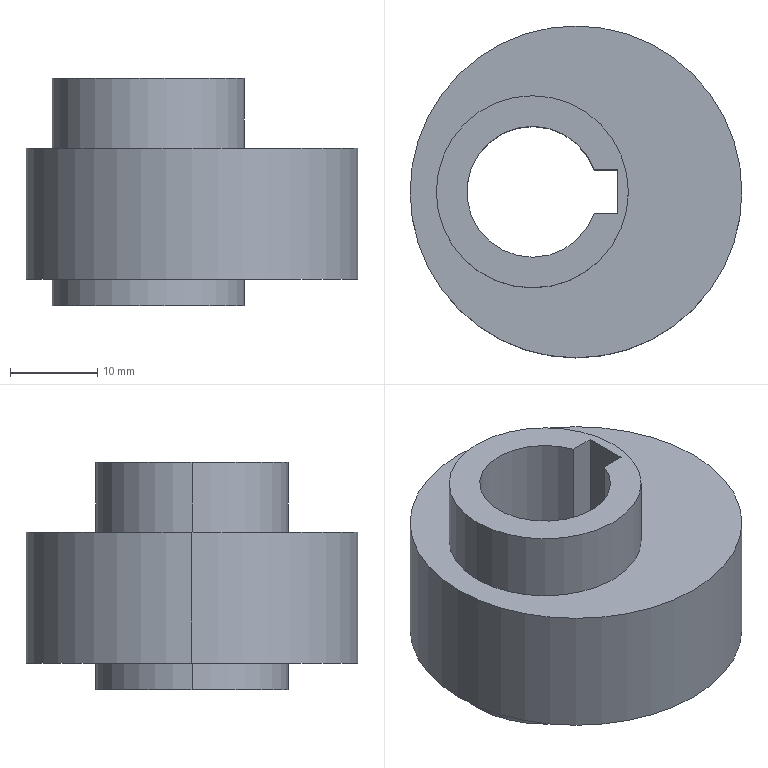Part | SolidWorks | features ICE 2, Extrusion 1 | 1 solid | 14 faces | box 38 x 38 x 26 mm | volume 16281 mm3 | cylinder 7 | plane 7 | commonest cylinder face diameters 22 x4 38 x2 15 x1
STEP:
#1=CARTESIAN_POINT('',(11.,0.,26.));
#2=VERTEX_POINT('',#1);
#3=CARTESIAN_POINT('',(-11.,0.,26.));
#4=VERTEX_POINT('',#3);
#5=CARTESIAN_POINT('',(0.,0.,26.));
#6=DIRECTION('',(0.,0.,1.));
#7=DIRECTION('',(1.,0.,0.));
#8=AXIS2_PLACEMENT_3D('',#5,#6,#7);
#9=CIRCLE('',#8,11.);
#10=EDGE_CURVE('',#2,#4,#9,.T.);
#11=ORIENTED_EDGE('',*,*,#10,.F.);
#12=CARTESIAN_POINT('',(11.,0.,18.));
#13=VERTEX_POINT('',#12);
#14=CARTESIAN_POINT('',(11.,0.,26.));
#15=DIRECTION('',(0.,0.,-1.));
#16=VECTOR('',#15,1000.);
#17=LINE('',#14,#16);
#18=EDGE_CURVE('',#2,#13,#17,.T.);
#19=ORIENTED_EDGE('',*,*,#18,.T.);
#20=CARTESIAN_POINT('',(-11.,0.,18.));
#21=VERTEX_POINT('',#20);
#22=CARTESIAN_POINT('',(0.,0.,18.));
#23=DIRECTION('',(0.,0.,1.));
#24=DIRECTION('',(1.,0.,0.));
#25=AXIS2_PLACEMENT_3D('',#22,#23,#24);
#26=CIRCLE('',#25,11.);
#27=EDGE_CURVE('',#13,#21,#26,.T.);
#28=ORIENTED_EDGE('',*,*,#27,.T.);
#29=CARTESIAN_POINT('',(-11.,0.,26.));
#30=DIRECTION('',(0.,0.,-1.));
#31=VECTOR('',#30,1000.);
#32=LINE('',#29,#31);
#33=EDGE_CURVE('',#4,#21,#32,.T.);
#34=ORIENTED_EDGE('',*,*,#33,.F.);
#35=EDGE_LOOP('',(#11,#19,#28,#34));
#36=FACE_OUTER_BOUND('',#35,.T.);
#37=CARTESIAN_POINT('',(0.,0.,26.));
#38=DIRECTION('',(0.,0.,-1.));
#39=DIRECTION('',(-1.,0.,0.));
#40=AXIS2_PLACEMENT_3D('',#37,#38,#39);
#41=CYLINDRICAL_SURFACE('',#40,11.);
#42=ADVANCED_FACE('',(#36),#41,.T.);
#43=CARTESIAN_POINT('',(24.,0.,3.));
#44=VERTEX_POINT('',#43);
#45=CARTESIAN_POINT('',(-14.,0.,3.));
#46=VERTEX_POINT('',#45);
#47=CARTESIAN_POINT('',(5.,0.,3.));
#48=DIRECTION('',(0.,0.,1.));
#49=DIRECTION('',(1.,0.,0.));
#50=AXIS2_PLACEMENT_3D('',#47,#48,#49);
#51=CIRCLE('',#50,19.);
#52=EDGE_CURVE('',#44,#46,#51,.T.);
#53=ORIENTED_EDGE('',*,*,#52,.T.);
#54=CARTESIAN_POINT('',(-14.,0.,18.));
#55=VERTEX_POINT('',#54);
#56=CARTESIAN_POINT('',(-14.,0.,3.));
#57=DIRECTION('',(0.,0.,1.));
#58=VECTOR('',#57,1000.);
#59=LINE('',#56,#58);
#60=EDGE_CURVE('',#46,#55,#59,.T.);
#61=ORIENTED_EDGE('',*,*,#60,.T.);
#62=CARTESIAN_POINT('',(24.,0.,18.));
#63=VERTEX_POINT('',#62);
#64=CARTESIAN_POINT('',(5.,0.,18.));
#65=DIRECTION('',(0.,0.,1.));
#66=DIRECTION('',(1.,0.,0.));
#67=AXIS2_PLACEMENT_3D('',#64,#65,#66);
#68=CIRCLE('',#67,19.);
#69=EDGE_CURVE('',#63,#55,#68,.T.);
#70=ORIENTED_EDGE('',*,*,#69,.F.);
#71=CARTESIAN_POINT('',(24.,0.,3.));
#72=DIRECTION('',(0.,0.,1.));
#73=VECTOR('',#72,1000.);
#74=LINE('',#71,#73);
#75=EDGE_CURVE('',#44,#63,#74,.T.);
#76=ORIENTED_EDGE('',*,*,#75,.F.);
#77=EDGE_LOOP('',(#53,#61,#70,#76));
#78=FACE_OUTER_BOUND('',#77,.T.);
#79=CARTESIAN_POINT('',(5.,0.,3.));
#80=DIRECTION('',(0.,0.,1.));
#81=DIRECTION('',(1.,0.,0.));
#82=AXIS2_PLACEMENT_3D('',#79,#80,#81);
#83=CYLINDRICAL_SURFACE('',#82,19.);
#84=ADVANCED_FACE('',(#78),#83,.T.);
#85=CARTESIAN_POINT('',(11.,0.,3.));
#86=VERTEX_POINT('',#85);
#87=CARTESIAN_POINT('',(-11.,0.,3.));
#88=VERTEX_POINT('',#87);
#89=CARTESIAN_POINT('',(0.,0.,3.));
#90=DIRECTION('',(0.,0.,1.));
#91=DIRECTION('',(1.,0.,0.));
#92=AXIS2_PLACEMENT_3D('',#89,#90,#91);
#93=CIRCLE('',#92,11.);
#94=EDGE_CURVE('',#86,#88,#93,.T.);
#95=ORIENTED_EDGE('',*,*,#94,.F.);
#96=CARTESIAN_POINT('',(11.,0.,0.));
#97=VERTEX_POINT('',#96);
#98=CARTESIAN_POINT('',(11.,0.,26.));
#99=DIRECTION('',(0.,0.,-1.));
#100=VECTOR('',#99,1000.);
#101=LINE('',#98,#100);
#102=EDGE_CURVE('',#86,#97,#101,.T.);
#103=ORIENTED_EDGE('',*,*,#102,.T.);
#104=CARTESIAN_POINT('',(-11.,0.,0.));
#105=VERTEX_POINT('',#104);
#106=CARTESIAN_POINT('',(0.,0.,0.));
#107=DIRECTION('',(0.,0.,1.));
#108=DIRECTION('',(1.,0.,0.));
#109=AXIS2_PLACEMENT_3D('',#106,#107,#108);
#110=CIRCLE('',#109,11.);
#111=EDGE_CURVE('',#97,#105,#110,.T.);
#112=ORIENTED_EDGE('',*,*,#111,.T.);
#113=CARTESIAN_POINT('',(-11.,0.,26.));
#114=DIRECTION('',(0.,0.,-1.));
#115=VECTOR('',#114,1000.);
#116=LINE('',#113,#115);
#117=EDGE_CURVE('',#88,#105,#116,.T.);
#118=ORIENTED_EDGE('',*,*,#117,.F.);
#119=EDGE_LOOP('',(#95,#103,#112,#118));
#120=FACE_OUTER_BOUND('',#119,.T.);
#121=CARTESIAN_POINT('',(0.,0.,26.));
#122=DIRECTION('',(0.,0.,-1.));
#123=DIRECTION('',(-1.,0.,0.));
#124=AXIS2_PLACEMENT_3D('',#121,#122,#123);
#125=CYLINDRICAL_SURFACE('',#124,11.);
#126=ADVANCED_FACE('',(#120),#125,.T.);
#127=ORIENTED_EDGE('',*,*,#102,.F.);
#128=CARTESIAN_POINT('',(0.,0.,3.));
#129=DIRECTION('',(0.,0.,1.));
#130=DIRECTION('',(1.,0.,0.));
#131=AXIS2_PLACEMENT_3D('',#128,#129,#130);
#132=CIRCLE('',#131,11.);
#133=EDGE_CURVE('',#88,#86,#132,.T.);
#134=ORIENTED_EDGE('',*,*,#133,.F.);
#135=ORIENTED_EDGE('',*,*,#117,.T.);
#136=CARTESIAN_POINT('',(0.,0.,0.));
#137=DIRECTION('',(0.,0.,1.));
#138=DIRECTION('',(1.,0.,0.));
#139=AXIS2_PLACEMENT_3D('',#136,#137,#138);
#140=CIRCLE('',#139,11.);
#141=EDGE_CURVE('',#105,#97,#140,.T.);
#142=ORIENTED_EDGE('',*,*,#141,.T.);
#143=EDGE_LOOP('',(#127,#134,#135,#142));
#144=FACE_OUTER_BOUND('',#143,.T.);
#145=CARTESIAN_POINT('',(0.,0.,26.));
#146=DIRECTION('',(0.,0.,-1.));
#147=DIRECTION('',(-1.,0.,0.));
#148=AXIS2_PLACEMENT_3D('',#145,#146,#147);
#149=CYLINDRICAL_SURFACE('',#148,11.);
#150=ADVANCED_FACE('',(#144),#149,.T.);
#151=CARTESIAN_POINT('',(9.8,2.5,0.));
#152=VERTEX_POINT('',#151);
#153=CARTESIAN_POINT('',(7.071,2.5,0.));
#154=VERTEX_POINT('',#153);
#155=CARTESIAN_POINT('',(0.,2.5,0.));
#156=DIRECTION('',(-1.,0.,0.));
#157=VECTOR('',#156,1000.);
#158=LINE('',#155,#157);
#159=EDGE_CURVE('',#152,#154,#158,.T.);
#160=ORIENTED_EDGE('',*,*,#159,.T.);
#161=CARTESIAN_POINT('',(7.071,-2.5,0.));
#162=VERTEX_POINT('',#161);
#163=CARTESIAN_POINT('',(0.,0.,0.));
#164=DIRECTION('',(0.,0.,1.));
#165=DIRECTION('',(1.,0.,0.));
#166=AXIS2_PLACEMENT_3D('',#163,#164,#165);
#167=CIRCLE('',#166,7.5);
#168=EDGE_CURVE('',#154,#162,#167,.T.);
#169=ORIENTED_EDGE('',*,*,#168,.T.);
#170=CARTESIAN_POINT('',(9.8,-2.5,0.));
#171=VERTEX_POINT('',#170);
#172=CARTESIAN_POINT('',(0.,-2.5,0.));
#173=DIRECTION('',(1.,0.,0.));
#174=VECTOR('',#173,1000.);
#175=LINE('',#172,#174);
#176=EDGE_CURVE('',#162,#171,#175,.T.);
#177=ORIENTED_EDGE('',*,*,#176,.T.);
#178=CARTESIAN_POINT('',(9.8,0.,0.));
#179=DIRECTION('',(0.,1.,0.));
#180=VECTOR('',#179,1000.);
#181=LINE('',#178,#180);
#182=EDGE_CURVE('',#171,#152,#181,.T.);
#183=ORIENTED_EDGE('',*,*,#182,.T.);
#184=EDGE_LOOP('',(#160,#169,#177,#183));
#185=FACE_BOUND('',#184,.T.);
#186=ORIENTED_EDGE('',*,*,#141,.F.);
#187=ORIENTED_EDGE('',*,*,#111,.F.);
#188=EDGE_LOOP('',(#186,#187));
#189=FACE_OUTER_BOUND('',#188,.T.);
#190=CARTESIAN_POINT('',(0.,0.,0.));
#191=DIRECTION('',(0.,0.,1.));
#192=DIRECTION('',(1.,0.,0.));
#193=AXIS2_PLACEMENT_3D('',#190,#191,#192);
#194=PLANE('',#193);
#195=ADVANCED_FACE('',(#185,#189),#194,.F.);
#196=ORIENTED_EDGE('',*,*,#60,.F.);
#197=CARTESIAN_POINT('',(5.,0.,3.));
#198=DIRECTION('',(0.,0.,1.));
#199=DIRECTION('',(1.,0.,0.));
#200=AXIS2_PLACEMENT_3D('',#197,#198,#199);
#201=CIRCLE('',#200,19.);
#202=EDGE_CURVE('',#46,#44,#201,.T.);
#203=ORIENTED_EDGE('',*,*,#202,.T.);
#204=ORIENTED_EDGE('',*,*,#75,.T.);
#205=CARTESIAN_POINT('',(5.,0.,18.));
#206=DIRECTION('',(0.,0.,1.));
#207=DIRECTION('',(1.,0.,0.));
#208=AXIS2_PLACEMENT_3D('',#205,#206,#207);
#209=CIRCLE('',#208,19.);
#210=EDGE_CURVE('',#55,#63,#209,.T.);
#211=ORIENTED_EDGE('',*,*,#210,.F.);
#212=EDGE_LOOP('',(#196,#203,#204,#211));
#213=FACE_OUTER_BOUND('',#212,.T.);
#214=CARTESIAN_POINT('',(5.,0.,3.));
#215=DIRECTION('',(0.,0.,1.));
#216=DIRECTION('',(1.,0.,0.));
#217=AXIS2_PLACEMENT_3D('',#214,#215,#216);
#218=CYLINDRICAL_SURFACE('',#217,19.);
#219=ADVANCED_FACE('',(#213),#218,.T.);
#220=ORIENTED_EDGE('',*,*,#133,.T.);
#221=ORIENTED_EDGE('',*,*,#94,.T.);
#222=EDGE_LOOP('',(#220,#221));
#223=FACE_BOUND('',#222,.T.);
#224=ORIENTED_EDGE('',*,*,#52,.F.);
#225=ORIENTED_EDGE('',*,*,#202,.F.);
#226=EDGE_LOOP('',(#224,#225));
#227=FACE_OUTER_BOUND('',#226,.T.);
#228=CARTESIAN_POINT('',(5.,0.,3.));
#229=DIRECTION('',(0.,0.,1.));
#230=DIRECTION('',(1.,0.,0.));
#231=AXIS2_PLACEMENT_3D('',#228,#229,#230);
#232=PLANE('',#231);
#233=ADVANCED_FACE('',(#223,#227),#232,.F.);
#234=CARTESIAN_POINT('',(0.,0.,18.));
#235=DIRECTION('',(0.,0.,1.));
#236=DIRECTION('',(1.,0.,0.));
#237=AXIS2_PLACEMENT_3D('',#234,#235,#236);
#238=CIRCLE('',#237,11.);
#239=EDGE_CURVE('',#21,#13,#238,.T.);
#240=ORIENTED_EDGE('',*,*,#239,.F.);
#241=ORIENTED_EDGE('',*,*,#27,.F.);
#242=EDGE_LOOP('',(#240,#241));
#243=FACE_BOUND('',#242,.T.);
#244=ORIENTED_EDGE('',*,*,#69,.T.);
#245=ORIENTED_EDGE('',*,*,#210,.T.);
#246=EDGE_LOOP('',(#244,#245));
#247=FACE_OUTER_BOUND('',#246,.T.);
#248=CARTESIAN_POINT('',(5.,0.,18.));
#249=DIRECTION('',(0.,0.,1.));
#250=DIRECTION('',(1.,0.,0.));
#251=AXIS2_PLACEMENT_3D('',#248,#249,#250);
#252=PLANE('',#251);
#253=ADVANCED_FACE('',(#243,#247),#252,.T.);
#254=CARTESIAN_POINT('',(7.071,2.5,26.));
#255=VERTEX_POINT('',#254);
#256=CARTESIAN_POINT('',(7.071,-2.5,26.));
#257=VERTEX_POINT('',#256);
#258=CARTESIAN_POINT('',(0.,0.,26.));
#259=DIRECTION('',(0.,0.,1.));
#260=DIRECTION('',(1.,0.,0.));
#261=AXIS2_PLACEMENT_3D('',#258,#259,#260);
#262=CIRCLE('',#261,7.5);
#263=EDGE_CURVE('',#255,#257,#262,.T.);
#264=ORIENTED_EDGE('',*,*,#263,.F.);
#265=CARTESIAN_POINT('',(9.8,2.5,26.));
#266=VERTEX_POINT('',#265);
#267=CARTESIAN_POINT('',(7.071,2.5,26.));
#268=DIRECTION('',(-1.,0.,0.));
#269=VECTOR('',#268,1000.);
#270=LINE('',#267,#269);
#271=EDGE_CURVE('',#266,#255,#270,.T.);
#272=ORIENTED_EDGE('',*,*,#271,.F.);
#273=CARTESIAN_POINT('',(9.8,-2.5,26.));
#274=VERTEX_POINT('',#273);
#275=CARTESIAN_POINT('',(9.8,2.5,26.));
#276=DIRECTION('',(0.,1.,0.));
#277=VECTOR('',#276,1000.);
#278=LINE('',#275,#277);
#279=EDGE_CURVE('',#274,#266,#278,.T.);
#280=ORIENTED_EDGE('',*,*,#279,.F.);
#281=CARTESIAN_POINT('',(9.8,-2.5,26.));
#282=DIRECTION('',(1.,0.,0.));
#283=VECTOR('',#282,1000.);
#284=LINE('',#281,#283);
#285=EDGE_CURVE('',#257,#274,#284,.T.);
#286=ORIENTED_EDGE('',*,*,#285,.F.);
#287=EDGE_LOOP('',(#264,#272,#280,#286));
#288=FACE_BOUND('',#287,.T.);
#289=CARTESIAN_POINT('',(0.,0.,26.));
#290=DIRECTION('',(0.,0.,1.));
#291=DIRECTION('',(1.,0.,0.));
#292=AXIS2_PLACEMENT_3D('',#289,#290,#291);
#293=CIRCLE('',#292,11.);
#294=EDGE_CURVE('',#4,#2,#293,.T.);
#295=ORIENTED_EDGE('',*,*,#294,.T.);
#296=ORIENTED_EDGE('',*,*,#10,.T.);
#297=EDGE_LOOP('',(#295,#296));
#298=FACE_OUTER_BOUND('',#297,.T.);
#299=CARTESIAN_POINT('',(0.,0.,26.));
#300=DIRECTION('',(0.,0.,1.));
#301=DIRECTION('',(1.,0.,0.));
#302=AXIS2_PLACEMENT_3D('',#299,#300,#301);
#303=PLANE('',#302);
#304=ADVANCED_FACE('',(#288,#298),#303,.T.);
#305=ORIENTED_EDGE('',*,*,#18,.F.);
#306=ORIENTED_EDGE('',*,*,#294,.F.);
#307=ORIENTED_EDGE('',*,*,#33,.T.);
#308=ORIENTED_EDGE('',*,*,#239,.T.);
#309=EDGE_LOOP('',(#305,#306,#307,#308));
#310=FACE_OUTER_BOUND('',#309,.T.);
#311=CARTESIAN_POINT('',(0.,0.,26.));
#312=DIRECTION('',(0.,0.,-1.));
#313=DIRECTION('',(-1.,0.,0.));
#314=AXIS2_PLACEMENT_3D('',#311,#312,#313);
#315=CYLINDRICAL_SURFACE('',#314,11.);
#316=ADVANCED_FACE('',(#310),#315,.T.);
#317=CARTESIAN_POINT('',(7.071,2.5,-17.));
#318=DIRECTION('',(0.,0.,1.));
#319=VECTOR('',#318,1000.);
#320=LINE('',#317,#319);
#321=EDGE_CURVE('',#154,#255,#320,.T.);
#322=ORIENTED_EDGE('',*,*,#321,.T.);
#323=ORIENTED_EDGE('',*,*,#263,.T.);
#324=CARTESIAN_POINT('',(7.071,-2.5,-17.));
#325=DIRECTION('',(0.,0.,1.));
#326=VECTOR('',#325,1000.);
#327=LINE('',#324,#326);
#328=EDGE_CURVE('',#162,#257,#327,.T.);
#329=ORIENTED_EDGE('',*,*,#328,.F.);
#330=ORIENTED_EDGE('',*,*,#168,.F.);
#331=EDGE_LOOP('',(#322,#323,#329,#330));
#332=FACE_OUTER_BOUND('',#331,.T.);
#333=CARTESIAN_POINT('',(0.,0.,-17.));
#334=DIRECTION('',(0.,0.,1.));
#335=DIRECTION('',(1.,0.,0.));
#336=AXIS2_PLACEMENT_3D('',#333,#334,#335);
#337=CYLINDRICAL_SURFACE('',#336,7.5);
#338=ADVANCED_FACE('',(#332),#337,.F.);
#339=CARTESIAN_POINT('',(9.8,2.5,-17.));
#340=DIRECTION('',(0.,0.,1.));
#341=VECTOR('',#340,1000.);
#342=LINE('',#339,#341);
#343=EDGE_CURVE('',#152,#266,#342,.T.);
#344=ORIENTED_EDGE('',*,*,#343,.T.);
#345=ORIENTED_EDGE('',*,*,#271,.T.);
#346=ORIENTED_EDGE('',*,*,#321,.F.);
#347=ORIENTED_EDGE('',*,*,#159,.F.);
#348=EDGE_LOOP('',(#344,#345,#346,#347));
#349=FACE_OUTER_BOUND('',#348,.T.);
#350=CARTESIAN_POINT('',(7.071,2.5,-17.));
#351=DIRECTION('',(0.,1.,0.));
#352=DIRECTION('',(-1.,0.,0.));
#353=AXIS2_PLACEMENT_3D('',#350,#351,#352);
#354=PLANE('',#353);
#355=ADVANCED_FACE('',(#349),#354,.F.);
#356=CARTESIAN_POINT('',(9.8,-2.5,-17.));
#357=DIRECTION('',(0.,0.,1.));
#358=VECTOR('',#357,1000.);
#359=LINE('',#356,#358);
#360=EDGE_CURVE('',#171,#274,#359,.T.);
#361=ORIENTED_EDGE('',*,*,#360,.T.);
#362=ORIENTED_EDGE('',*,*,#279,.T.);
#363=ORIENTED_EDGE('',*,*,#343,.F.);
#364=ORIENTED_EDGE('',*,*,#182,.F.);
#365=EDGE_LOOP('',(#361,#362,#363,#364));
#366=FACE_OUTER_BOUND('',#365,.T.);
#367=CARTESIAN_POINT('',(9.8,2.5,-17.));
#368=DIRECTION('',(1.,0.,0.));
#369=DIRECTION('',(0.,0.,-1.));
#370=AXIS2_PLACEMENT_3D('',#367,#368,#369);
#371=PLANE('',#370);
#372=ADVANCED_FACE('',(#366),#371,.F.);
#373=ORIENTED_EDGE('',*,*,#328,.T.);
#374=ORIENTED_EDGE('',*,*,#285,.T.);
#375=ORIENTED_EDGE('',*,*,#360,.F.);
#376=ORIENTED_EDGE('',*,*,#176,.F.);
#377=EDGE_LOOP('',(#373,#374,#375,#376));
#378=FACE_OUTER_BOUND('',#377,.T.);
#379=CARTESIAN_POINT('',(9.8,-2.5,-17.));
#380=DIRECTION('',(0.,-1.,0.));
#381=DIRECTION('',(1.,0.,0.));
#382=AXIS2_PLACEMENT_3D('',#379,#380,#381);
#383=PLANE('',#382);
#384=ADVANCED_FACE('',(#378),#383,.F.);
#385=CLOSED_SHELL('',(#42,#84,#126,#150,#195,#219,#233,#253,#304,#316,#338,#355,#372,#384));
#386=MANIFOLD_SOLID_BREP('',#385);
#387=CARTESIAN_POINT('',(0.,0.,0.));
#388=DIRECTION('',(0.,0.,1.));
#389=DIRECTION('',(1.,0.,0.));
#390=AXIS2_PLACEMENT_3D('',#387,#388,#389);
#391=(LENGTH_UNIT()NAMED_UNIT(*)SI_UNIT(.MILLI.,.METRE.));
#392=UNCERTAINTY_MEASURE_WITH_UNIT(LENGTH_MEASURE(0.00001),#391,'','');
#393=(NAMED_UNIT(*)PLANE_ANGLE_UNIT()SI_UNIT($,.RADIAN.));
#394=(NAMED_UNIT(*)SI_UNIT($,.STERADIAN.)SOLID_ANGLE_UNIT());
#395=(GEOMETRIC_REPRESENTATION_CONTEXT(3)GLOBAL_UNCERTAINTY_ASSIGNED_CONTEXT((#392))GLOBAL_UNIT_ASSIGNED_CONTEXT((#391,#393,#394))REPRESENTATION_CONTEXT('',''));
#396=ADVANCED_BREP_SHAPE_REPRESENTATION('',(#386,#390),#395);